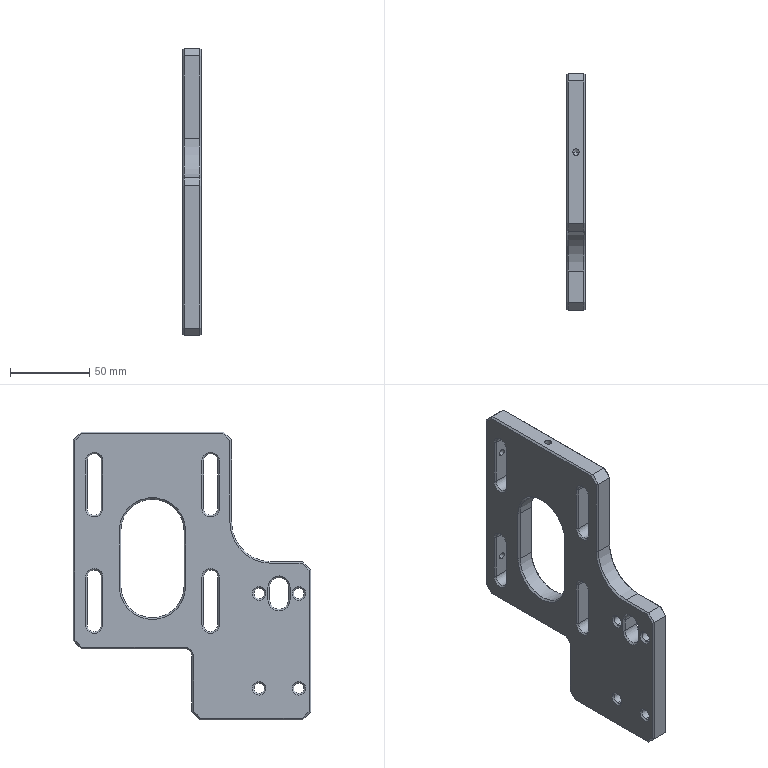Part | SolidWorks | features BaseBody 1 | 1 solid | 167 faces | box 12 x 150 x 182 mm | volume 184850 mm3 | plane 80 | cone 53 | cylinder 34 | commonest cylinder face diameters 9 x12 6.6 x8 4.2 x6 12 x3 40 x3 10 x1